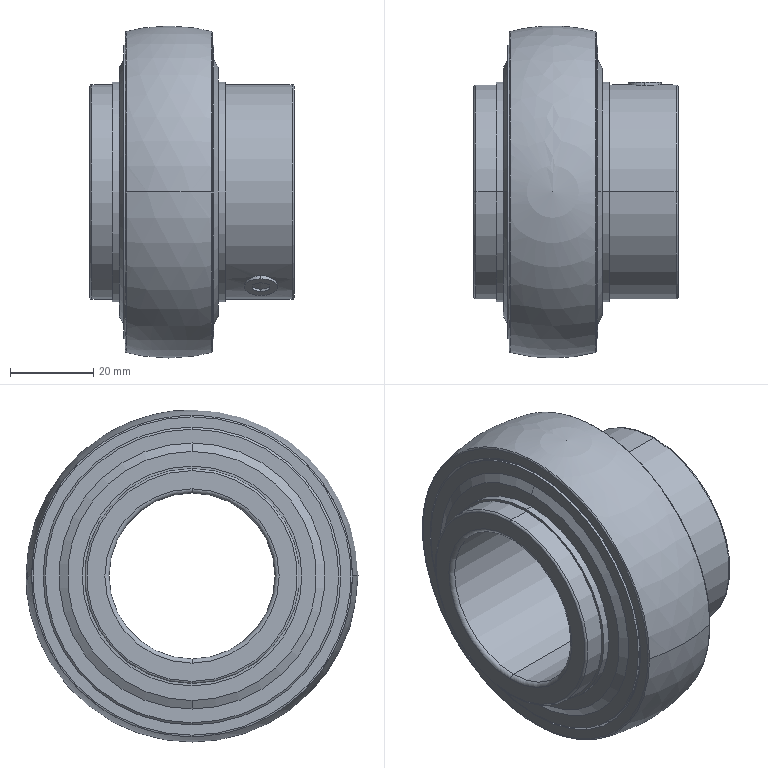Part | SolidWorks | features BaseBody 1 | 1 solid | 184 faces | box 49.2 x 80 x 80 mm | volume 69188 mm3 | cone 60 | cylinder 46 | plane 42 | torus 34 | sphere 2 | commonest cylinder face diameters 51.8 x14 8 x4 52.96 x4 53.03 x4 53.645 x4 69.842 x4